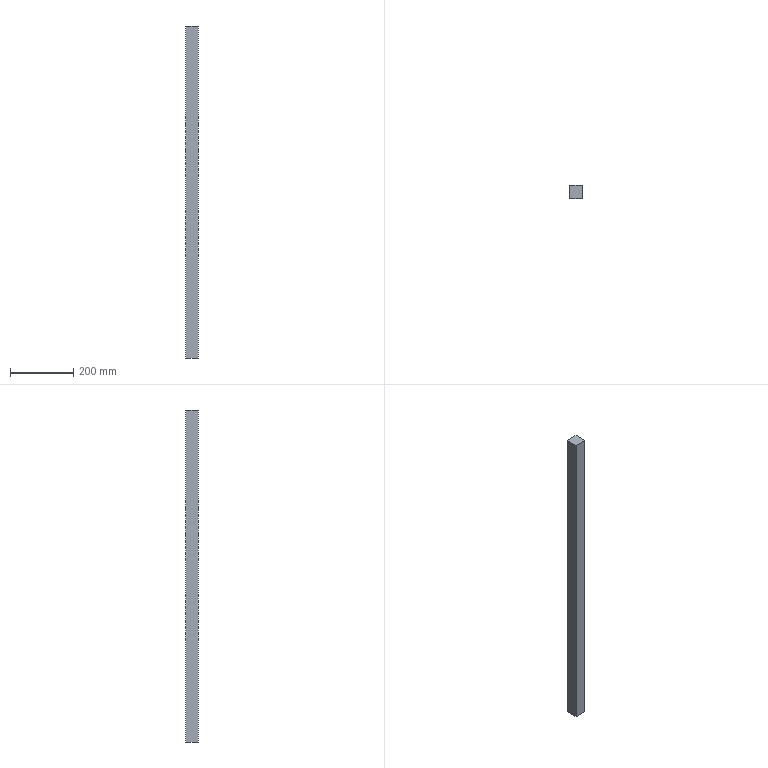Part | NX | features 凸台-拉伸7 2 | 1 solid | 6 faces | box 40 x 40 x 1050 mm | volume 1680000 mm3 | plane 6
STEP:
#1=CARTESIAN_POINT('',(973.,-560.,-12.985));
#2=VERTEX_POINT('',#1);
#3=CARTESIAN_POINT('',(933.,-560.,-12.985));
#4=VERTEX_POINT('',#3);
#5=CARTESIAN_POINT('',(933.,-560.,-12.985));
#6=DIRECTION('',(-1.,0.,0.));
#7=VECTOR('',#6,1000.);
#8=LINE('',#5,#7);
#9=EDGE_CURVE('',#2,#4,#8,.T.);
#10=ORIENTED_EDGE('',*,*,#9,.T.);
#11=CARTESIAN_POINT('',(933.,-600.,-12.985));
#12=VERTEX_POINT('',#11);
#13=CARTESIAN_POINT('',(933.,-600.,-12.985));
#14=DIRECTION('',(0.,-1.,0.));
#15=VECTOR('',#14,1000.);
#16=LINE('',#13,#15);
#17=EDGE_CURVE('',#4,#12,#16,.T.);
#18=ORIENTED_EDGE('',*,*,#17,.T.);
#19=CARTESIAN_POINT('',(973.,-600.,-12.985));
#20=VERTEX_POINT('',#19);
#21=CARTESIAN_POINT('',(933.,-600.,-12.985));
#22=DIRECTION('',(1.,0.,0.));
#23=VECTOR('',#22,1000.);
#24=LINE('',#21,#23);
#25=EDGE_CURVE('',#12,#20,#24,.T.);
#26=ORIENTED_EDGE('',*,*,#25,.T.);
#27=CARTESIAN_POINT('',(973.,-600.,-12.985));
#28=DIRECTION('',(0.,1.,0.));
#29=VECTOR('',#28,1000.);
#30=LINE('',#27,#29);
#31=EDGE_CURVE('',#20,#2,#30,.T.);
#32=ORIENTED_EDGE('',*,*,#31,.T.);
#33=EDGE_LOOP('',(#10,#18,#26,#32));
#34=FACE_BOUND('',#33,.T.);
#35=CARTESIAN_POINT('',(1349.569,-600.,-12.985));
#36=DIRECTION('',(0.,0.,1.));
#37=DIRECTION('',(1.,0.,0.));
#38=AXIS2_PLACEMENT_3D('',#35,#36,#37);
#39=PLANE('',#38);
#40=ADVANCED_FACE('',(#34),#39,.T.);
#41=CARTESIAN_POINT('',(933.,-560.,-1062.985));
#42=VERTEX_POINT('',#41);
#43=CARTESIAN_POINT('',(933.,-600.,-1062.985));
#44=VERTEX_POINT('',#43);
#45=CARTESIAN_POINT('',(933.,-600.,-1062.985));
#46=DIRECTION('',(0.,-1.,0.));
#47=VECTOR('',#46,1000.);
#48=LINE('',#45,#47);
#49=EDGE_CURVE('',#42,#44,#48,.T.);
#50=ORIENTED_EDGE('',*,*,#49,.F.);
#51=CARTESIAN_POINT('',(973.,-560.,-1062.985));
#52=VERTEX_POINT('',#51);
#53=CARTESIAN_POINT('',(933.,-560.,-1062.985));
#54=DIRECTION('',(-1.,0.,0.));
#55=VECTOR('',#54,1000.);
#56=LINE('',#53,#55);
#57=EDGE_CURVE('',#52,#42,#56,.T.);
#58=ORIENTED_EDGE('',*,*,#57,.F.);
#59=CARTESIAN_POINT('',(973.,-600.,-1062.985));
#60=VERTEX_POINT('',#59);
#61=CARTESIAN_POINT('',(973.,-600.,-1062.985));
#62=DIRECTION('',(0.,1.,0.));
#63=VECTOR('',#62,1000.);
#64=LINE('',#61,#63);
#65=EDGE_CURVE('',#60,#52,#64,.T.);
#66=ORIENTED_EDGE('',*,*,#65,.F.);
#67=CARTESIAN_POINT('',(933.,-600.,-1062.985));
#68=DIRECTION('',(1.,0.,0.));
#69=VECTOR('',#68,1000.);
#70=LINE('',#67,#69);
#71=EDGE_CURVE('',#44,#60,#70,.T.);
#72=ORIENTED_EDGE('',*,*,#71,.F.);
#73=EDGE_LOOP('',(#50,#58,#66,#72));
#74=FACE_BOUND('',#73,.T.);
#75=CARTESIAN_POINT('',(0.,0.,-1062.985));
#76=DIRECTION('',(0.,0.,-1.));
#77=DIRECTION('',(-1.,0.,0.));
#78=AXIS2_PLACEMENT_3D('',#75,#76,#77);
#79=PLANE('',#78);
#80=ADVANCED_FACE('',(#74),#79,.T.);
#81=ORIENTED_EDGE('',*,*,#9,.F.);
#82=CARTESIAN_POINT('',(973.,-560.,43.584));
#83=DIRECTION('',(0.,0.,-1.));
#84=VECTOR('',#83,1000.);
#85=LINE('',#82,#84);
#86=EDGE_CURVE('',#2,#52,#85,.T.);
#87=ORIENTED_EDGE('',*,*,#86,.T.);
#88=ORIENTED_EDGE('',*,*,#57,.T.);
#89=CARTESIAN_POINT('',(933.,-560.,43.584));
#90=DIRECTION('',(0.,0.,-1.));
#91=VECTOR('',#90,1000.);
#92=LINE('',#89,#91);
#93=EDGE_CURVE('',#4,#42,#92,.T.);
#94=ORIENTED_EDGE('',*,*,#93,.F.);
#95=EDGE_LOOP('',(#81,#87,#88,#94));
#96=FACE_BOUND('',#95,.T.);
#97=CARTESIAN_POINT('',(933.,-560.,43.584));
#98=DIRECTION('',(0.,-1.,0.));
#99=DIRECTION('',(0.,0.,-1.));
#100=AXIS2_PLACEMENT_3D('',#97,#98,#99);
#101=PLANE('',#100);
#102=ADVANCED_FACE('',(#96),#101,.F.);
#103=ORIENTED_EDGE('',*,*,#31,.F.);
#104=CARTESIAN_POINT('',(973.,-600.,43.584));
#105=DIRECTION('',(0.,0.,-1.));
#106=VECTOR('',#105,1000.);
#107=LINE('',#104,#106);
#108=EDGE_CURVE('',#20,#60,#107,.T.);
#109=ORIENTED_EDGE('',*,*,#108,.T.);
#110=ORIENTED_EDGE('',*,*,#65,.T.);
#111=ORIENTED_EDGE('',*,*,#86,.F.);
#112=EDGE_LOOP('',(#103,#109,#110,#111));
#113=FACE_BOUND('',#112,.T.);
#114=CARTESIAN_POINT('',(973.,-600.,43.584));
#115=DIRECTION('',(-1.,0.,0.));
#116=DIRECTION('',(0.,0.,1.));
#117=AXIS2_PLACEMENT_3D('',#114,#115,#116);
#118=PLANE('',#117);
#119=ADVANCED_FACE('',(#113),#118,.F.);
#120=ORIENTED_EDGE('',*,*,#25,.F.);
#121=CARTESIAN_POINT('',(933.,-600.,43.584));
#122=DIRECTION('',(0.,0.,-1.));
#123=VECTOR('',#122,1000.);
#124=LINE('',#121,#123);
#125=EDGE_CURVE('',#12,#44,#124,.T.);
#126=ORIENTED_EDGE('',*,*,#125,.T.);
#127=ORIENTED_EDGE('',*,*,#71,.T.);
#128=ORIENTED_EDGE('',*,*,#108,.F.);
#129=EDGE_LOOP('',(#120,#126,#127,#128));
#130=FACE_BOUND('',#129,.T.);
#131=CARTESIAN_POINT('',(933.,-600.,43.584));
#132=DIRECTION('',(0.,1.,0.));
#133=DIRECTION('',(0.,0.,1.));
#134=AXIS2_PLACEMENT_3D('',#131,#132,#133);
#135=PLANE('',#134);
#136=ADVANCED_FACE('',(#130),#135,.F.);
#137=ORIENTED_EDGE('',*,*,#17,.F.);
#138=ORIENTED_EDGE('',*,*,#93,.T.);
#139=ORIENTED_EDGE('',*,*,#49,.T.);
#140=ORIENTED_EDGE('',*,*,#125,.F.);
#141=EDGE_LOOP('',(#137,#138,#139,#140));
#142=FACE_BOUND('',#141,.T.);
#143=CARTESIAN_POINT('',(933.,-600.,43.584));
#144=DIRECTION('',(1.,0.,0.));
#145=DIRECTION('',(0.,0.,-1.));
#146=AXIS2_PLACEMENT_3D('',#143,#144,#145);
#147=PLANE('',#146);
#148=ADVANCED_FACE('',(#142),#147,.F.);
#149=CLOSED_SHELL('',(#40,#80,#102,#119,#136,#148));
#150=MANIFOLD_SOLID_BREP('',#149);
#151=(LENGTH_UNIT()NAMED_UNIT(*)SI_UNIT(.MILLI.,.METRE.));
#152=UNCERTAINTY_MEASURE_WITH_UNIT(LENGTH_MEASURE(0.00001),#151,'','');
#153=(NAMED_UNIT(*)PLANE_ANGLE_UNIT()SI_UNIT($,.RADIAN.));
#154=(NAMED_UNIT(*)SI_UNIT($,.STERADIAN.)SOLID_ANGLE_UNIT());
#155=(GEOMETRIC_REPRESENTATION_CONTEXT(3)GLOBAL_UNCERTAINTY_ASSIGNED_CONTEXT((#152))GLOBAL_UNIT_ASSIGNED_CONTEXT((#151,#153,#154))REPRESENTATION_CONTEXT('',''));
#156=ADVANCED_BREP_SHAPE_REPRESENTATION('',(#150),#155);